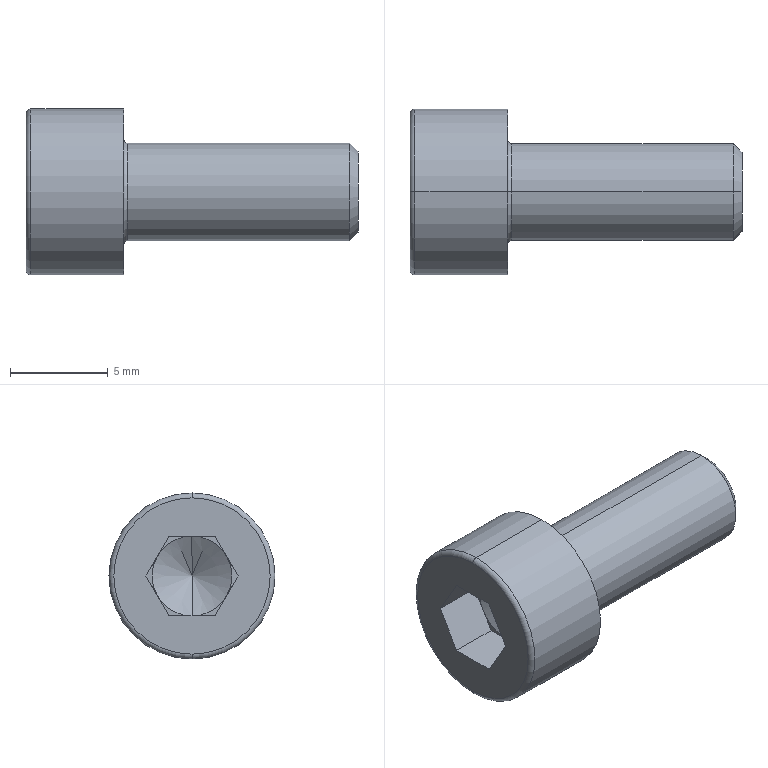Part | STEP file | socket head cap screw_iso_ISO 4762 M5 x 12 --- 12N | 1 solid | 27 faces | box 17 x 8.5 x 8.5 mm | volume 476.406 mm3 | plane 15 | cone 4 | torus 4 | cylinder 4 | commonest cylinder face diameters 5 x2 8.5 x2